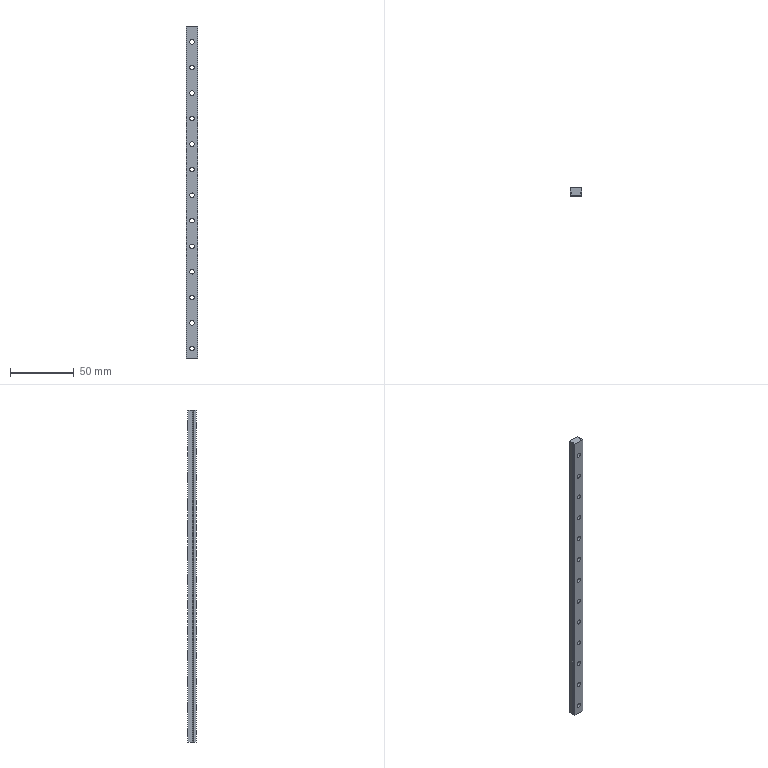Part | SolidWorks | features BaseBody 1 | 1 solid | 79 faces | box 9 x 6.5 x 260 mm | volume 12909 mm3 | cylinder 52 | plane 27 | commonest cylinder face diameters 3.5 x26 6.5 x26